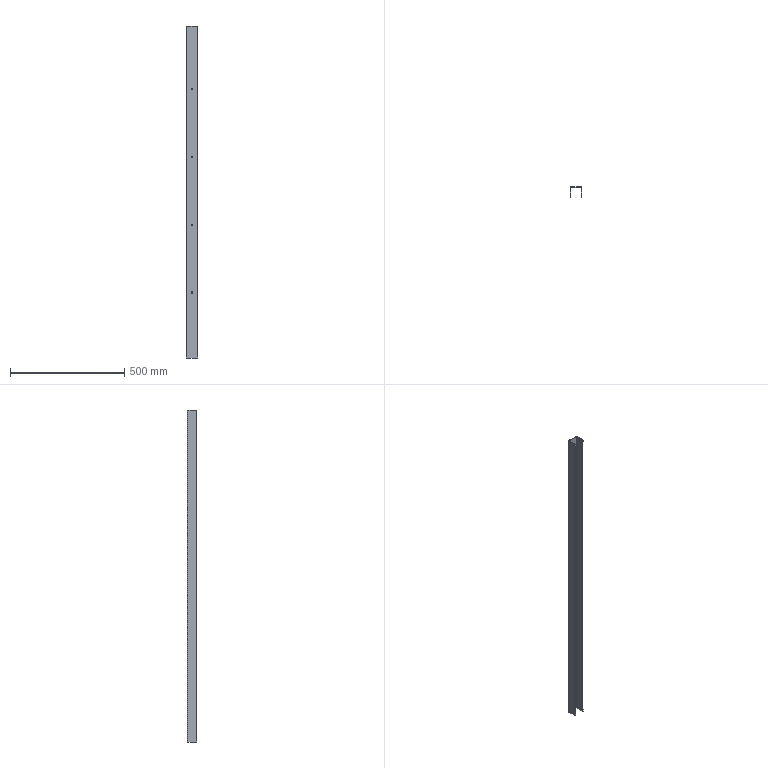Part | STEP file | SX-004-10 | 1 solid | 38 faces | box 50 x 41.5 x 1450 mm | volume 359516 mm3 | plane 26 | cylinder 12 | commonest cylinder face diameters 5 x8 0.4 x2 4.4 x2